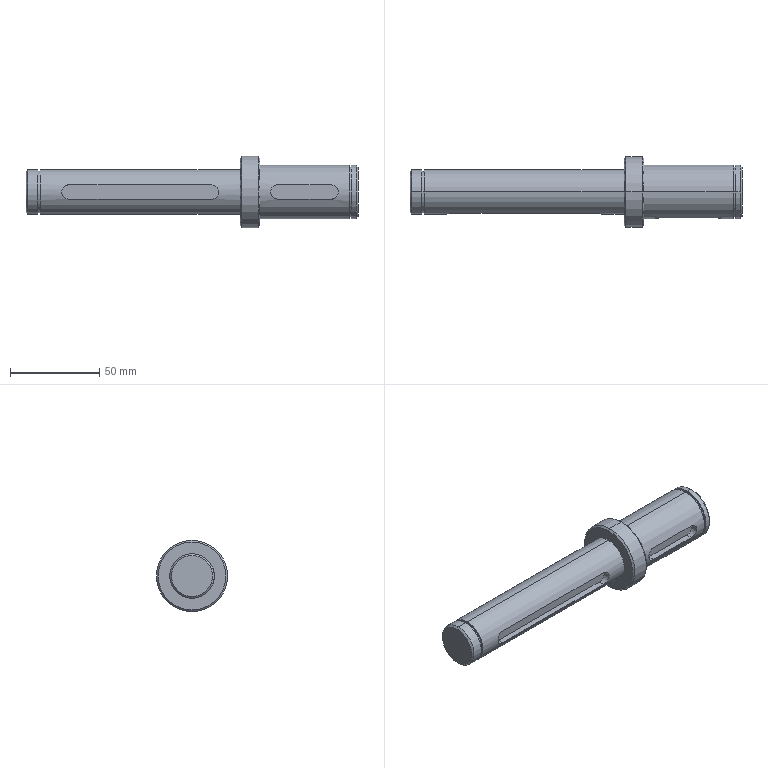Part | STEP file | 4-Rotating drive shaft | 1 solid | 40 faces | box 186 x 40 x 40 mm | volume 107459 mm3 | cylinder 18 | plane 14 | cone 8 | commonest cylinder face diameters 8 x4 25 x4 30 x4 23.2 x2 27.9 x2 40 x2